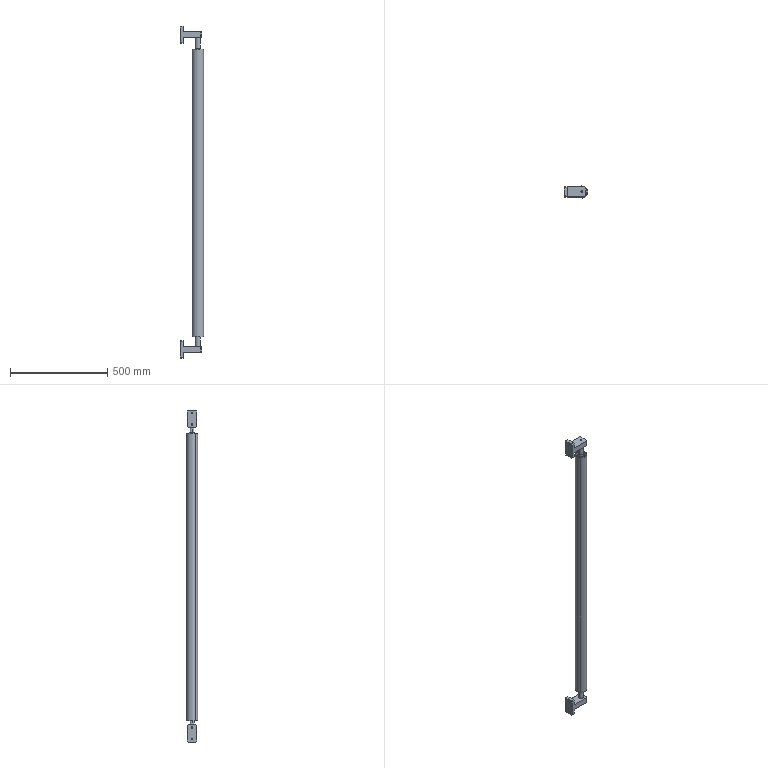Part | SolidWorks | 6 solids | 334 faces | box 120 x 60 x 1710 mm | volume 2689604 mm3 | torus 124 | cylinder 70 | sphere 68 | plane 56 | cone 16 | commonest cylinder face diameters 9 x12 25 x10 15 x8 23 x8 29 x8 6.8 x4